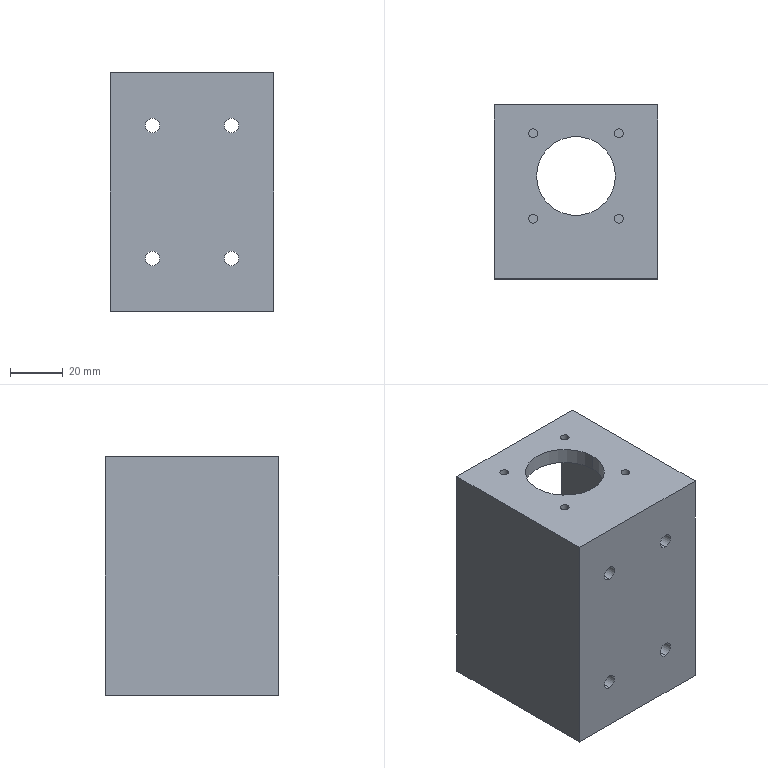Part | Creo | features CURVE 7, CUT 4, DATUM PLANE 3, PROTRUSION 2, CHAMFER 1, COORDINATE SYSTEM 1 | 1 solid | 45 faces | box 62 x 66 x 90.5 mm | volume 126268 mm3 | cylinder 26 | plane 19 | commonest cylinder face diameters 3.3 x8 5.5 x8 4.2 x6 30 x2 34 x2
STEP:
#1=CARTESIAN_POINT('',(0.,0.,0.));
#2=DIRECTION('',(0.,0.,1.));
#3=DIRECTION('',(1.,0.,0.));
#4=AXIS2_PLACEMENT_3D('',#1,#2,#3);
#5=CARTESIAN_POINT('',(31.,27.,0.));
#6=VERTEX_POINT('',#5);
#7=CARTESIAN_POINT('',(-31.,27.,0.));
#8=VERTEX_POINT('',#7);
#9=CARTESIAN_POINT('',(31.,27.,0.));
#10=DIRECTION('',(-1.,0.,0.));
#11=VECTOR('',#10,62.);
#12=LINE('',#9,#11);
#13=EDGE_CURVE('',#6,#8,#12,.T.);
#14=ORIENTED_EDGE('',*,*,#13,.T.);
#15=CARTESIAN_POINT('',(-31.,-39.,0.));
#16=VERTEX_POINT('',#15);
#17=CARTESIAN_POINT('',(-31.,27.,0.));
#18=DIRECTION('',(0.,-1.,0.));
#19=VECTOR('',#18,66.);
#20=LINE('',#17,#19);
#21=EDGE_CURVE('',#8,#16,#20,.T.);
#22=ORIENTED_EDGE('',*,*,#21,.T.);
#23=CARTESIAN_POINT('',(31.,-39.,0.));
#24=VERTEX_POINT('',#23);
#25=CARTESIAN_POINT('',(-31.,-39.,0.));
#26=DIRECTION('',(1.,0.,0.));
#27=VECTOR('',#26,62.);
#28=LINE('',#25,#27);
#29=EDGE_CURVE('',#16,#24,#28,.T.);
#30=ORIENTED_EDGE('',*,*,#29,.T.);
#31=CARTESIAN_POINT('',(31.,-39.,0.));
#32=DIRECTION('',(0.,1.,0.));
#33=VECTOR('',#32,66.);
#34=LINE('',#31,#33);
#35=EDGE_CURVE('',#24,#6,#34,.T.);
#36=ORIENTED_EDGE('',*,*,#35,.T.);
#37=EDGE_LOOP('',(#14,#22,#30,#36));
#38=FACE_OUTER_BOUND('',#37,.F.);
#39=CARTESIAN_POINT('',(0.,-17.,0.));
#40=VERTEX_POINT('',#39);
#41=CARTESIAN_POINT('',(0.,17.,0.));
#42=VERTEX_POINT('',#41);
#43=CARTESIAN_POINT('',(0.,0.,0.));
#44=DIRECTION('',(0.,0.,-1.));
#45=DIRECTION('',(0.,-1.,0.));
#46=AXIS2_PLACEMENT_3D('',#43,#44,#45);
#47=CIRCLE('',#46,17.);
#48=EDGE_CURVE('',#40,#42,#47,.T.);
#49=ORIENTED_EDGE('',*,*,#48,.T.);
#50=CARTESIAN_POINT('',(0.,0.,0.));
#51=DIRECTION('',(0.,0.,-1.));
#52=DIRECTION('',(0.,1.,0.));
#53=AXIS2_PLACEMENT_3D('',#50,#51,#52);
#54=CIRCLE('',#53,17.);
#55=EDGE_CURVE('',#42,#40,#54,.T.);
#56=ORIENTED_EDGE('',*,*,#55,.T.);
#57=EDGE_LOOP('',(#49,#56));
#58=FACE_BOUND('',#57,.F.);
#59=CARTESIAN_POINT('',(0.,18.9,0.));
#60=VERTEX_POINT('',#59);
#61=CARTESIAN_POINT('',(0.,23.1,0.));
#62=VERTEX_POINT('',#61);
#63=CARTESIAN_POINT('',(0.,21.,0.));
#64=DIRECTION('',(0.,0.,-1.));
#65=DIRECTION('',(0.,-1.,0.));
#66=AXIS2_PLACEMENT_3D('',#63,#64,#65);
#67=CIRCLE('',#66,2.1);
#68=EDGE_CURVE('',#60,#62,#67,.T.);
#69=ORIENTED_EDGE('',*,*,#68,.T.);
#70=CARTESIAN_POINT('',(0.,21.,0.));
#71=DIRECTION('',(0.,0.,-1.));
#72=DIRECTION('',(0.,1.,0.));
#73=AXIS2_PLACEMENT_3D('',#70,#71,#72);
#74=CIRCLE('',#73,2.1);
#75=EDGE_CURVE('',#62,#60,#74,.T.);
#76=ORIENTED_EDGE('',*,*,#75,.T.);
#77=EDGE_LOOP('',(#69,#76));
#78=FACE_BOUND('',#77,.F.);
#79=CARTESIAN_POINT('',(-18.187,-12.6,0.));
#80=VERTEX_POINT('',#79);
#81=CARTESIAN_POINT('',(-18.187,-8.4,0.));
#82=VERTEX_POINT('',#81);
#83=CARTESIAN_POINT('',(-18.187,-10.5,0.));
#84=DIRECTION('',(0.,0.,-1.));
#85=DIRECTION('',(0.,-1.,0.));
#86=AXIS2_PLACEMENT_3D('',#83,#84,#85);
#87=CIRCLE('',#86,2.1);
#88=EDGE_CURVE('',#80,#82,#87,.T.);
#89=ORIENTED_EDGE('',*,*,#88,.T.);
#90=CARTESIAN_POINT('',(-18.187,-10.5,0.));
#91=DIRECTION('',(0.,0.,-1.));
#92=DIRECTION('',(0.,1.,0.));
#93=AXIS2_PLACEMENT_3D('',#90,#91,#92);
#94=CIRCLE('',#93,2.1);
#95=EDGE_CURVE('',#82,#80,#94,.T.);
#96=ORIENTED_EDGE('',*,*,#95,.T.);
#97=EDGE_LOOP('',(#89,#96));
#98=FACE_BOUND('',#97,.F.);
#99=CARTESIAN_POINT('',(18.187,-12.6,0.));
#100=VERTEX_POINT('',#99);
#101=CARTESIAN_POINT('',(18.187,-8.4,0.));
#102=VERTEX_POINT('',#101);
#103=CARTESIAN_POINT('',(18.187,-10.5,0.));
#104=DIRECTION('',(0.,0.,-1.));
#105=DIRECTION('',(0.,-1.,0.));
#106=AXIS2_PLACEMENT_3D('',#103,#104,#105);
#107=CIRCLE('',#106,2.1);
#108=EDGE_CURVE('',#100,#102,#107,.T.);
#109=ORIENTED_EDGE('',*,*,#108,.T.);
#110=CARTESIAN_POINT('',(18.187,-10.5,0.));
#111=DIRECTION('',(0.,0.,-1.));
#112=DIRECTION('',(0.,1.,0.));
#113=AXIS2_PLACEMENT_3D('',#110,#111,#112);
#114=CIRCLE('',#113,2.1);
#115=EDGE_CURVE('',#102,#100,#114,.T.);
#116=ORIENTED_EDGE('',*,*,#115,.T.);
#117=EDGE_LOOP('',(#109,#116));
#118=FACE_BOUND('',#117,.F.);
#119=CARTESIAN_POINT('',(0.,0.,0.));
#120=DIRECTION('',(0.,0.,1.));
#121=DIRECTION('',(1.,0.,0.));
#122=AXIS2_PLACEMENT_3D('',#119,#120,#121);
#123=PLANE('',#122);
#124=ADVANCED_FACE('',(#38,#58,#78,#98,#118),#123,.F.);
#125=ORIENTED_EDGE('',*,*,#13,.F.);
#126=CARTESIAN_POINT('',(31.,27.,90.5));
#127=VERTEX_POINT('',#126);
#128=CARTESIAN_POINT('',(31.,27.,0.));
#129=DIRECTION('',(0.,0.,1.));
#130=VECTOR('',#129,90.5);
#131=LINE('',#128,#130);
#132=EDGE_CURVE('',#6,#127,#131,.T.);
#133=ORIENTED_EDGE('',*,*,#132,.T.);
#134=CARTESIAN_POINT('',(-31.,27.,90.5));
#135=VERTEX_POINT('',#134);
#136=CARTESIAN_POINT('',(31.,27.,90.5));
#137=DIRECTION('',(-1.,0.,0.));
#138=VECTOR('',#137,62.);
#139=LINE('',#136,#138);
#140=EDGE_CURVE('',#127,#135,#139,.T.);
#141=ORIENTED_EDGE('',*,*,#140,.T.);
#142=CARTESIAN_POINT('',(-31.,27.,0.));
#143=DIRECTION('',(0.,0.,1.));
#144=VECTOR('',#143,90.5);
#145=LINE('',#142,#144);
#146=EDGE_CURVE('',#8,#135,#145,.T.);
#147=ORIENTED_EDGE('',*,*,#146,.F.);
#148=EDGE_LOOP('',(#125,#133,#141,#147));
#149=FACE_OUTER_BOUND('',#148,.F.);
#150=CARTESIAN_POINT('',(-25.,27.,9.));
#151=VERTEX_POINT('',#150);
#152=CARTESIAN_POINT('',(-25.,27.,81.5));
#153=VERTEX_POINT('',#152);
#154=CARTESIAN_POINT('',(-25.,27.,9.));
#155=DIRECTION('',(0.,0.,1.));
#156=VECTOR('',#155,72.5);
#157=LINE('',#154,#156);
#158=EDGE_CURVE('',#151,#153,#157,.T.);
#159=ORIENTED_EDGE('',*,*,#158,.T.);
#160=CARTESIAN_POINT('',(-22.,27.,84.5));
#161=VERTEX_POINT('',#160);
#162=CARTESIAN_POINT('',(-22.,27.,84.5));
#163=DIRECTION('',(-0.7071,0.,-0.7071));
#164=VECTOR('',#163,4.243);
#165=LINE('',#162,#164);
#166=EDGE_CURVE('',#161,#153,#165,.T.);
#167=ORIENTED_EDGE('',*,*,#166,.F.);
#168=CARTESIAN_POINT('',(22.,27.,84.5));
#169=VERTEX_POINT('',#168);
#170=CARTESIAN_POINT('',(-22.,27.,84.5));
#171=DIRECTION('',(1.,0.,0.));
#172=VECTOR('',#171,44.);
#173=LINE('',#170,#172);
#174=EDGE_CURVE('',#161,#169,#173,.T.);
#175=ORIENTED_EDGE('',*,*,#174,.T.);
#176=CARTESIAN_POINT('',(25.,27.,81.5));
#177=VERTEX_POINT('',#176);
#178=CARTESIAN_POINT('',(25.,27.,81.5));
#179=DIRECTION('',(-0.7071,0.,0.7071));
#180=VECTOR('',#179,4.243);
#181=LINE('',#178,#180);
#182=EDGE_CURVE('',#177,#169,#181,.T.);
#183=ORIENTED_EDGE('',*,*,#182,.F.);
#184=CARTESIAN_POINT('',(25.,27.,9.));
#185=VERTEX_POINT('',#184);
#186=CARTESIAN_POINT('',(25.,27.,81.5));
#187=DIRECTION('',(0.,0.,-1.));
#188=VECTOR('',#187,72.5);
#189=LINE('',#186,#188);
#190=EDGE_CURVE('',#177,#185,#189,.T.);
#191=ORIENTED_EDGE('',*,*,#190,.T.);
#192=CARTESIAN_POINT('',(22.,27.,6.));
#193=VERTEX_POINT('',#192);
#194=CARTESIAN_POINT('',(22.,27.,6.));
#195=DIRECTION('',(0.7071,0.,0.7071));
#196=VECTOR('',#195,4.243);
#197=LINE('',#194,#196);
#198=EDGE_CURVE('',#193,#185,#197,.T.);
#199=ORIENTED_EDGE('',*,*,#198,.F.);
#200=CARTESIAN_POINT('',(-22.,27.,6.));
#201=VERTEX_POINT('',#200);
#202=CARTESIAN_POINT('',(22.,27.,6.));
#203=DIRECTION('',(-1.,0.,0.));
#204=VECTOR('',#203,44.);
#205=LINE('',#202,#204);
#206=EDGE_CURVE('',#193,#201,#205,.T.);
#207=ORIENTED_EDGE('',*,*,#206,.T.);
#208=CARTESIAN_POINT('',(-25.,27.,9.));
#209=DIRECTION('',(0.7071,0.,-0.7071));
#210=VECTOR('',#209,4.243);
#211=LINE('',#208,#210);
#212=EDGE_CURVE('',#151,#201,#211,.T.);
#213=ORIENTED_EDGE('',*,*,#212,.F.);
#214=EDGE_LOOP('',(#159,#167,#175,#183,#191,#199,#207,#213));
#215=FACE_BOUND('',#214,.F.);
#216=CARTESIAN_POINT('',(31.,27.,0.));
#217=DIRECTION('',(0.,1.,0.));
#218=DIRECTION('',(-1.,0.,0.));
#219=AXIS2_PLACEMENT_3D('',#216,#217,#218);
#220=PLANE('',#219);
#221=ADVANCED_FACE('',(#149,#215),#220,.T.);
#222=ORIENTED_EDGE('',*,*,#35,.F.);
#223=CARTESIAN_POINT('',(31.,-39.,90.5));
#224=VERTEX_POINT('',#223);
#225=CARTESIAN_POINT('',(31.,-39.,0.));
#226=DIRECTION('',(0.,0.,1.));
#227=VECTOR('',#226,90.5);
#228=LINE('',#225,#227);
#229=EDGE_CURVE('',#24,#224,#228,.T.);
#230=ORIENTED_EDGE('',*,*,#229,.T.);
#231=CARTESIAN_POINT('',(31.,-39.,90.5));
#232=DIRECTION('',(0.,1.,0.));
#233=VECTOR('',#232,66.);
#234=LINE('',#231,#233);
#235=EDGE_CURVE('',#224,#127,#234,.T.);
#236=ORIENTED_EDGE('',*,*,#235,.T.);
#237=ORIENTED_EDGE('',*,*,#132,.F.);
#238=EDGE_LOOP('',(#222,#230,#236,#237));
#239=FACE_OUTER_BOUND('',#238,.F.);
#240=CARTESIAN_POINT('',(31.,-39.,0.));
#241=DIRECTION('',(1.,0.,0.));
#242=DIRECTION('',(0.,1.,0.));
#243=AXIS2_PLACEMENT_3D('',#240,#241,#242);
#244=PLANE('',#243);
#245=ADVANCED_FACE('',(#239),#244,.T.);
#246=ORIENTED_EDGE('',*,*,#29,.F.);
#247=CARTESIAN_POINT('',(-31.,-39.,90.5));
#248=VERTEX_POINT('',#247);
#249=CARTESIAN_POINT('',(-31.,-39.,0.));
#250=DIRECTION('',(0.,0.,1.));
#251=VECTOR('',#250,90.5);
#252=LINE('',#249,#251);
#253=EDGE_CURVE('',#16,#248,#252,.T.);
#254=ORIENTED_EDGE('',*,*,#253,.T.);
#255=CARTESIAN_POINT('',(-31.,-39.,90.5));
#256=DIRECTION('',(1.,0.,0.));
#257=VECTOR('',#256,62.);
#258=LINE('',#255,#257);
#259=EDGE_CURVE('',#248,#224,#258,.T.);
#260=ORIENTED_EDGE('',*,*,#259,.T.);
#261=ORIENTED_EDGE('',*,*,#229,.F.);
#262=EDGE_LOOP('',(#246,#254,#260,#261));
#263=FACE_OUTER_BOUND('',#262,.F.);
#264=CARTESIAN_POINT('',(-15.,-39.,67.75));
#265=VERTEX_POINT('',#264);
#266=CARTESIAN_POINT('',(-15.,-39.,73.25));
#267=VERTEX_POINT('',#266);
#268=CARTESIAN_POINT('',(-15.,-39.,70.5));
#269=DIRECTION('',(0.,1.,0.));
#270=DIRECTION('',(0.,0.,-1.));
#271=AXIS2_PLACEMENT_3D('',#268,#269,#270);
#272=CIRCLE('',#271,2.75);
#273=EDGE_CURVE('',#265,#267,#272,.T.);
#274=ORIENTED_EDGE('',*,*,#273,.F.);
#275=CARTESIAN_POINT('',(-15.,-39.,70.5));
#276=DIRECTION('',(0.,1.,0.));
#277=DIRECTION('',(0.,0.,1.));
#278=AXIS2_PLACEMENT_3D('',#275,#276,#277);
#279=CIRCLE('',#278,2.75);
#280=EDGE_CURVE('',#267,#265,#279,.T.);
#281=ORIENTED_EDGE('',*,*,#280,.F.);
#282=EDGE_LOOP('',(#274,#281));
#283=FACE_BOUND('',#282,.F.);
#284=CARTESIAN_POINT('',(-15.,-39.,17.25));
#285=VERTEX_POINT('',#284);
#286=CARTESIAN_POINT('',(-15.,-39.,22.75));
#287=VERTEX_POINT('',#286);
#288=CARTESIAN_POINT('',(-15.,-39.,20.));
#289=DIRECTION('',(0.,1.,0.));
#290=DIRECTION('',(0.,0.,-1.));
#291=AXIS2_PLACEMENT_3D('',#288,#289,#290);
#292=CIRCLE('',#291,2.75);
#293=EDGE_CURVE('',#285,#287,#292,.T.);
#294=ORIENTED_EDGE('',*,*,#293,.F.);
#295=CARTESIAN_POINT('',(-15.,-39.,20.));
#296=DIRECTION('',(0.,1.,0.));
#297=DIRECTION('',(0.,0.,1.));
#298=AXIS2_PLACEMENT_3D('',#295,#296,#297);
#299=CIRCLE('',#298,2.75);
#300=EDGE_CURVE('',#287,#285,#299,.T.);
#301=ORIENTED_EDGE('',*,*,#300,.F.);
#302=EDGE_LOOP('',(#294,#301));
#303=FACE_BOUND('',#302,.F.);
#304=CARTESIAN_POINT('',(15.,-39.,17.25));
#305=VERTEX_POINT('',#304);
#306=CARTESIAN_POINT('',(15.,-39.,22.75));
#307=VERTEX_POINT('',#306);
#308=CARTESIAN_POINT('',(15.,-39.,20.));
#309=DIRECTION('',(0.,1.,0.));
#310=DIRECTION('',(0.,0.,-1.));
#311=AXIS2_PLACEMENT_3D('',#308,#309,#310);
#312=CIRCLE('',#311,2.75);
#313=EDGE_CURVE('',#305,#307,#312,.T.);
#314=ORIENTED_EDGE('',*,*,#313,.F.);
#315=CARTESIAN_POINT('',(15.,-39.,20.));
#316=DIRECTION('',(0.,1.,0.));
#317=DIRECTION('',(0.,0.,1.));
#318=AXIS2_PLACEMENT_3D('',#315,#316,#317);
#319=CIRCLE('',#318,2.75);
#320=EDGE_CURVE('',#307,#305,#319,.T.);
#321=ORIENTED_EDGE('',*,*,#320,.F.);
#322=EDGE_LOOP('',(#314,#321));
#323=FACE_BOUND('',#322,.F.);
#324=CARTESIAN_POINT('',(15.,-39.,67.75));
#325=VERTEX_POINT('',#324);
#326=CARTESIAN_POINT('',(15.,-39.,73.25));
#327=VERTEX_POINT('',#326);
#328=CARTESIAN_POINT('',(15.,-39.,70.5));
#329=DIRECTION('',(0.,1.,0.));
#330=DIRECTION('',(0.,0.,-1.));
#331=AXIS2_PLACEMENT_3D('',#328,#329,#330);
#332=CIRCLE('',#331,2.75);
#333=EDGE_CURVE('',#325,#327,#332,.T.);
#334=ORIENTED_EDGE('',*,*,#333,.F.);
#335=CARTESIAN_POINT('',(15.,-39.,70.5));
#336=DIRECTION('',(0.,1.,0.));
#337=DIRECTION('',(0.,0.,1.));
#338=AXIS2_PLACEMENT_3D('',#335,#336,#337);
#339=CIRCLE('',#338,2.75);
#340=EDGE_CURVE('',#327,#325,#339,.T.);
#341=ORIENTED_EDGE('',*,*,#340,.F.);
#342=EDGE_LOOP('',(#334,#341));
#343=FACE_BOUND('',#342,.F.);
#344=CARTESIAN_POINT('',(-31.,-39.,0.));
#345=DIRECTION('',(0.,-1.,0.));
#346=DIRECTION('',(1.,0.,0.));
#347=AXIS2_PLACEMENT_3D('',#344,#345,#346);
#348=PLANE('',#347);
#349=ADVANCED_FACE('',(#263,#283,#303,#323,#343),#348,.T.);
#350=ORIENTED_EDGE('',*,*,#21,.F.);
#351=ORIENTED_EDGE('',*,*,#146,.T.);
#352=CARTESIAN_POINT('',(-31.,27.,90.5));
#353=DIRECTION('',(0.,-1.,0.));
#354=VECTOR('',#353,66.);
#355=LINE('',#352,#354);
#356=EDGE_CURVE('',#135,#248,#355,.T.);
#357=ORIENTED_EDGE('',*,*,#356,.T.);
#358=ORIENTED_EDGE('',*,*,#253,.F.);
#359=EDGE_LOOP('',(#350,#351,#357,#358));
#360=FACE_OUTER_BOUND('',#359,.F.);
#361=CARTESIAN_POINT('',(-31.,27.,0.));
#362=DIRECTION('',(-1.,0.,0.));
#363=DIRECTION('',(0.,-1.,0.));
#364=AXIS2_PLACEMENT_3D('',#361,#362,#363);
#365=PLANE('',#364);
#366=ADVANCED_FACE('',(#360),#365,.T.);
#367=ORIENTED_EDGE('',*,*,#140,.F.);
#368=ORIENTED_EDGE('',*,*,#235,.F.);
#369=ORIENTED_EDGE('',*,*,#259,.F.);
#370=ORIENTED_EDGE('',*,*,#356,.F.);
#371=EDGE_LOOP('',(#367,#368,#369,#370));
#372=FACE_OUTER_BOUND('',#371,.F.);
#373=CARTESIAN_POINT('',(-14.61,16.26,90.5));
#374=VERTEX_POINT('',#373);
#375=CARTESIAN_POINT('',(-17.91,16.26,90.5));
#376=VERTEX_POINT('',#375);
#377=CARTESIAN_POINT('',(-16.26,16.26,90.5));
#378=DIRECTION('',(0.,0.,-1.));
#379=DIRECTION('',(1.,0.,0.));
#380=AXIS2_PLACEMENT_3D('',#377,#378,#379);
#381=CIRCLE('',#380,1.65);
#382=EDGE_CURVE('',#374,#376,#381,.T.);
#383=ORIENTED_EDGE('',*,*,#382,.F.);
#384=CARTESIAN_POINT('',(-16.26,16.26,90.5));
#385=DIRECTION('',(0.,0.,-1.));
#386=DIRECTION('',(-1.,0.,0.));
#387=AXIS2_PLACEMENT_3D('',#384,#385,#386);
#388=CIRCLE('',#387,1.65);
#389=EDGE_CURVE('',#376,#374,#388,.T.);
#390=ORIENTED_EDGE('',*,*,#389,.F.);
#391=EDGE_LOOP('',(#383,#390));
#392=FACE_BOUND('',#391,.F.);
#393=CARTESIAN_POINT('',(17.91,16.26,90.5));
#394=VERTEX_POINT('',#393);
#395=CARTESIAN_POINT('',(14.61,16.26,90.5));
#396=VERTEX_POINT('',#395);
#397=CARTESIAN_POINT('',(16.26,16.26,90.5));
#398=DIRECTION('',(0.,0.,-1.));
#399=DIRECTION('',(1.,0.,0.));
#400=AXIS2_PLACEMENT_3D('',#397,#398,#399);
#401=CIRCLE('',#400,1.65);
#402=EDGE_CURVE('',#394,#396,#401,.T.);
#403=ORIENTED_EDGE('',*,*,#402,.F.);
#404=CARTESIAN_POINT('',(16.26,16.26,90.5));
#405=DIRECTION('',(0.,0.,-1.));
#406=DIRECTION('',(-1.,0.,0.));
#407=AXIS2_PLACEMENT_3D('',#404,#405,#406);
#408=CIRCLE('',#407,1.65);
#409=EDGE_CURVE('',#396,#394,#408,.T.);
#410=ORIENTED_EDGE('',*,*,#409,.F.);
#411=EDGE_LOOP('',(#403,#410));
#412=FACE_BOUND('',#411,.F.);
#413=CARTESIAN_POINT('',(17.91,-16.26,90.5));
#414=VERTEX_POINT('',#413);
#415=CARTESIAN_POINT('',(14.61,-16.26,90.5));
#416=VERTEX_POINT('',#415);
#417=CARTESIAN_POINT('',(16.26,-16.26,90.5));
#418=DIRECTION('',(0.,0.,-1.));
#419=DIRECTION('',(1.,0.,0.));
#420=AXIS2_PLACEMENT_3D('',#417,#418,#419);
#421=CIRCLE('',#420,1.65);
#422=EDGE_CURVE('',#414,#416,#421,.T.);
#423=ORIENTED_EDGE('',*,*,#422,.F.);
#424=CARTESIAN_POINT('',(16.26,-16.26,90.5));
#425=DIRECTION('',(0.,0.,-1.));
#426=DIRECTION('',(-1.,0.,0.));
#427=AXIS2_PLACEMENT_3D('',#424,#425,#426);
#428=CIRCLE('',#427,1.65);
#429=EDGE_CURVE('',#416,#414,#428,.T.);
#430=ORIENTED_EDGE('',*,*,#429,.F.);
#431=EDGE_LOOP('',(#423,#430));
#432=FACE_BOUND('',#431,.F.);
#433=CARTESIAN_POINT('',(-14.61,-16.26,90.5));
#434=VERTEX_POINT('',#433);
#435=CARTESIAN_POINT('',(-17.91,-16.26,90.5));
#436=VERTEX_POINT('',#435);
#437=CARTESIAN_POINT('',(-16.26,-16.26,90.5));
#438=DIRECTION('',(0.,0.,-1.));
#439=DIRECTION('',(1.,0.,0.));
#440=AXIS2_PLACEMENT_3D('',#437,#438,#439);
#441=CIRCLE('',#440,1.65);
#442=EDGE_CURVE('',#434,#436,#441,.T.);
#443=ORIENTED_EDGE('',*,*,#442,.F.);
#444=CARTESIAN_POINT('',(-16.26,-16.26,90.5));
#445=DIRECTION('',(0.,0.,-1.));
#446=DIRECTION('',(-1.,0.,0.));
#447=AXIS2_PLACEMENT_3D('',#444,#445,#446);
#448=CIRCLE('',#447,1.65);
#449=EDGE_CURVE('',#436,#434,#448,.T.);
#450=ORIENTED_EDGE('',*,*,#449,.F.);
#451=EDGE_LOOP('',(#443,#450));
#452=FACE_BOUND('',#451,.F.);
#453=CARTESIAN_POINT('',(15.,0.,90.5));
#454=VERTEX_POINT('',#453);
#455=CARTESIAN_POINT('',(-15.,0.,90.5));
#456=VERTEX_POINT('',#455);
#457=CARTESIAN_POINT('',(0.,0.,90.5));
#458=DIRECTION('',(0.,0.,-1.));
#459=DIRECTION('',(1.,0.,0.));
#460=AXIS2_PLACEMENT_3D('',#457,#458,#459);
#461=CIRCLE('',#460,15.);
#462=EDGE_CURVE('',#454,#456,#461,.T.);
#463=ORIENTED_EDGE('',*,*,#462,.F.);
#464=CARTESIAN_POINT('',(0.,0.,90.5));
#465=DIRECTION('',(0.,0.,-1.));
#466=DIRECTION('',(-1.,0.,0.));
#467=AXIS2_PLACEMENT_3D('',#464,#465,#466);
#468=CIRCLE('',#467,15.);
#469=EDGE_CURVE('',#456,#454,#468,.T.);
#470=ORIENTED_EDGE('',*,*,#469,.F.);
#471=EDGE_LOOP('',(#463,#470));
#472=FACE_BOUND('',#471,.F.);
#473=CARTESIAN_POINT('',(0.,0.,90.5));
#474=DIRECTION('',(0.,0.,1.));
#475=DIRECTION('',(1.,0.,0.));
#476=AXIS2_PLACEMENT_3D('',#473,#474,#475);
#477=PLANE('',#476);
#478=ADVANCED_FACE('',(#372,#392,#412,#432,#452,#472),#477,.T.);
#479=CARTESIAN_POINT('',(-15.,0.,84.5));
#480=VERTEX_POINT('',#479);
#481=CARTESIAN_POINT('',(15.,0.,84.5));
#482=VERTEX_POINT('',#481);
#483=CARTESIAN_POINT('',(0.,0.,84.5));
#484=DIRECTION('',(0.,0.,1.));
#485=DIRECTION('',(-1.,0.,0.));
#486=AXIS2_PLACEMENT_3D('',#483,#484,#485);
#487=CIRCLE('',#486,15.);
#488=EDGE_CURVE('',#480,#482,#487,.T.);
#489=ORIENTED_EDGE('',*,*,#488,.T.);
#490=CARTESIAN_POINT('',(15.,0.,84.5));
#491=DIRECTION('',(0.,0.,1.));
#492=VECTOR('',#491,6.);
#493=LINE('',#490,#492);
#494=EDGE_CURVE('',#482,#454,#493,.T.);
#495=ORIENTED_EDGE('',*,*,#494,.T.);
#496=ORIENTED_EDGE('',*,*,#462,.T.);
#497=CARTESIAN_POINT('',(-15.,0.,84.5));
#498=DIRECTION('',(0.,0.,1.));
#499=VECTOR('',#498,6.);
#500=LINE('',#497,#499);
#501=EDGE_CURVE('',#480,#456,#500,.T.);
#502=ORIENTED_EDGE('',*,*,#501,.F.);
#503=EDGE_LOOP('',(#489,#495,#496,#502));
#504=FACE_OUTER_BOUND('',#503,.F.);
#505=CARTESIAN_POINT('',(0.,0.,0.));
#506=DIRECTION('',(0.,0.,1.));
#507=DIRECTION('',(1.,0.,0.));
#508=AXIS2_PLACEMENT_3D('',#505,#506,#507);
#509=CYLINDRICAL_SURFACE('',#508,15.);
#510=ADVANCED_FACE('',(#504),#509,.F.);
#511=CARTESIAN_POINT('',(22.,-30.,84.5));
#512=VERTEX_POINT('',#511);
#513=CARTESIAN_POINT('',(22.,27.,84.5));
#514=DIRECTION('',(0.,-1.,0.));
#515=VECTOR('',#514,57.);
#516=LINE('',#513,#515);
#517=EDGE_CURVE('',#169,#512,#516,.T.);
#518=ORIENTED_EDGE('',*,*,#517,.F.);
#519=ORIENTED_EDGE('',*,*,#174,.F.);
#520=CARTESIAN_POINT('',(-22.,-30.,84.5));
#521=VERTEX_POINT('',#520);
#522=CARTESIAN_POINT('',(-22.,27.,84.5));
#523=DIRECTION('',(0.,-1.,0.));
#524=VECTOR('',#523,57.);
#525=LINE('',#522,#524);
#526=EDGE_CURVE('',#161,#521,#525,.T.);
#527=ORIENTED_EDGE('',*,*,#526,.T.);
#528=CARTESIAN_POINT('',(22.,-30.,84.5));
#529=DIRECTION('',(-1.,0.,0.));
#530=VECTOR('',#529,44.);
#531=LINE('',#528,#530);
#532=EDGE_CURVE('',#512,#521,#531,.T.);
#533=ORIENTED_EDGE('',*,*,#532,.F.);
#534=EDGE_LOOP('',(#518,#519,#527,#533));
#535=FACE_OUTER_BOUND('',#534,.F.);
#536=CARTESIAN_POINT('',(-17.91,16.26,84.5));
#537=VERTEX_POINT('',#536);
#538=CARTESIAN_POINT('',(-14.61,16.26,84.5));
#539=VERTEX_POINT('',#538);
#540=CARTESIAN_POINT('',(-16.26,16.26,84.5));
#541=DIRECTION('',(0.,0.,1.));
#542=DIRECTION('',(-1.,0.,0.));
#543=AXIS2_PLACEMENT_3D('',#540,#541,#542);
#544=CIRCLE('',#543,1.65);
#545=EDGE_CURVE('',#537,#539,#544,.T.);
#546=ORIENTED_EDGE('',*,*,#545,.F.);
#547=CARTESIAN_POINT('',(-16.26,16.26,84.5));
#548=DIRECTION('',(0.,0.,1.));
#549=DIRECTION('',(1.,0.,0.));
#550=AXIS2_PLACEMENT_3D('',#547,#548,#549);
#551=CIRCLE('',#550,1.65);
#552=EDGE_CURVE('',#539,#537,#551,.T.);
#553=ORIENTED_EDGE('',*,*,#552,.F.);
#554=EDGE_LOOP('',(#546,#553));
#555=FACE_BOUND('',#554,.F.);
#556=CARTESIAN_POINT('',(14.61,16.26,84.5));
#557=VERTEX_POINT('',#556);
#558=CARTESIAN_POINT('',(17.91,16.26,84.5));
#559=VERTEX_POINT('',#558);
#560=CARTESIAN_POINT('',(16.26,16.26,84.5));
#561=DIRECTION('',(0.,0.,1.));
#562=DIRECTION('',(-1.,0.,0.));
#563=AXIS2_PLACEMENT_3D('',#560,#561,#562);
#564=CIRCLE('',#563,1.65);
#565=EDGE_CURVE('',#557,#559,#564,.T.);
#566=ORIENTED_EDGE('',*,*,#565,.F.);
#567=CARTESIAN_POINT('',(16.26,16.26,84.5));
#568=DIRECTION('',(0.,0.,1.));
#569=DIRECTION('',(1.,0.,0.));
#570=AXIS2_PLACEMENT_3D('',#567,#568,#569);
#571=CIRCLE('',#570,1.65);
#572=EDGE_CURVE('',#559,#557,#571,.T.);
#573=ORIENTED_EDGE('',*,*,#572,.F.);
#574=EDGE_LOOP('',(#566,#573));
#575=FACE_BOUND('',#574,.F.);
#576=CARTESIAN_POINT('',(14.61,-16.26,84.5));
#577=VERTEX_POINT('',#576);
#578=CARTESIAN_POINT('',(17.91,-16.26,84.5));
#579=VERTEX_POINT('',#578);
#580=CARTESIAN_POINT('',(16.26,-16.26,84.5));
#581=DIRECTION('',(0.,0.,1.));
#582=DIRECTION('',(-1.,0.,0.));
#583=AXIS2_PLACEMENT_3D('',#580,#581,#582);
#584=CIRCLE('',#583,1.65);
#585=EDGE_CURVE('',#577,#579,#584,.T.);
#586=ORIENTED_EDGE('',*,*,#585,.F.);
#587=CARTESIAN_POINT('',(16.26,-16.26,84.5));
#588=DIRECTION('',(0.,0.,1.));
#589=DIRECTION('',(1.,0.,0.));
#590=AXIS2_PLACEMENT_3D('',#587,#588,#589);
#591=CIRCLE('',#590,1.65);
#592=EDGE_CURVE('',#579,#577,#591,.T.);
#593=ORIENTED_EDGE('',*,*,#592,.F.);
#594=EDGE_LOOP('',(#586,#593));
#595=FACE_BOUND('',#594,.F.);
#596=CARTESIAN_POINT('',(-17.91,-16.26,84.5));
#597=VERTEX_POINT('',#596);
#598=CARTESIAN_POINT('',(-14.61,-16.26,84.5));
#599=VERTEX_POINT('',#598);
#600=CARTESIAN_POINT('',(-16.26,-16.26,84.5));
#601=DIRECTION('',(0.,0.,1.));
#602=DIRECTION('',(-1.,0.,0.));
#603=AXIS2_PLACEMENT_3D('',#600,#601,#602);
#604=CIRCLE('',#603,1.65);
#605=EDGE_CURVE('',#597,#599,#604,.T.);
#606=ORIENTED_EDGE('',*,*,#605,.F.);
#607=CARTESIAN_POINT('',(-16.26,-16.26,84.5));
#608=DIRECTION('',(0.,0.,1.));
#609=DIRECTION('',(1.,0.,0.));
#610=AXIS2_PLACEMENT_3D('',#607,#608,#609);
#611=CIRCLE('',#610,1.65);
#612=EDGE_CURVE('',#599,#597,#611,.T.);
#613=ORIENTED_EDGE('',*,*,#612,.F.);
#614=EDGE_LOOP('',(#606,#613));
#615=FACE_BOUND('',#614,.F.);
#616=ORIENTED_EDGE('',*,*,#488,.F.);
#617=CARTESIAN_POINT('',(0.,0.,84.5));
#618=DIRECTION('',(0.,0.,1.));
#619=DIRECTION('',(1.,0.,0.));
#620=AXIS2_PLACEMENT_3D('',#617,#618,#619);
#621=CIRCLE('',#620,15.);
#622=EDGE_CURVE('',#482,#480,#621,.T.);
#623=ORIENTED_EDGE('',*,*,#622,.F.);
#624=EDGE_LOOP('',(#616,#623));
#625=FACE_BOUND('',#624,.F.);
#626=CARTESIAN_POINT('',(-25.,27.,84.5));
#627=DIRECTION('',(0.,0.,1.));
#628=DIRECTION('',(1.,0.,0.));
#629=AXIS2_PLACEMENT_3D('',#626,#627,#628);
#630=PLANE('',#629);
#631=ADVANCED_FACE('',(#535,#555,#575,#595,#615,#625),#630,.F.);
#632=ORIENTED_EDGE('',*,*,#622,.T.);
#633=ORIENTED_EDGE('',*,*,#501,.T.);
#634=ORIENTED_EDGE('',*,*,#469,.T.);
#635=ORIENTED_EDGE('',*,*,#494,.F.);
#636=EDGE_LOOP('',(#632,#633,#634,#635));
#637=FACE_OUTER_BOUND('',#636,.F.);
#638=CARTESIAN_POINT('',(0.,0.,0.));
#639=DIRECTION('',(0.,0.,1.));
#640=DIRECTION('',(1.,0.,0.));
#641=AXIS2_PLACEMENT_3D('',#638,#639,#640);
#642=CYLINDRICAL_SURFACE('',#641,15.);
#643=ADVANCED_FACE('',(#637),#642,.F.);
#644=ORIENTED_EDGE('',*,*,#545,.T.);
#645=CARTESIAN_POINT('',(-14.61,16.26,84.5));
#646=DIRECTION('',(0.,0.,1.));
#647=VECTOR('',#646,6.);
#648=LINE('',#645,#647);
#649=EDGE_CURVE('',#539,#374,#648,.T.);
#650=ORIENTED_EDGE('',*,*,#649,.T.);
#651=ORIENTED_EDGE('',*,*,#382,.T.);
#652=CARTESIAN_POINT('',(-17.91,16.26,84.5));
#653=DIRECTION('',(0.,0.,1.));
#654=VECTOR('',#653,6.);
#655=LINE('',#652,#654);
#656=EDGE_CURVE('',#537,#376,#655,.T.);
#657=ORIENTED_EDGE('',*,*,#656,.F.);
#658=EDGE_LOOP('',(#644,#650,#651,#657));
#659=FACE_OUTER_BOUND('',#658,.F.);
#660=CARTESIAN_POINT('',(-16.26,16.26,0.));
#661=DIRECTION('',(0.,0.,1.));
#662=DIRECTION('',(1.,0.,0.));
#663=AXIS2_PLACEMENT_3D('',#660,#661,#662);
#664=CYLINDRICAL_SURFACE('',#663,1.65);
#665=ADVANCED_FACE('',(#659),#664,.F.);
#666=ORIENTED_EDGE('',*,*,#552,.T.);
#667=ORIENTED_EDGE('',*,*,#656,.T.);
#668=ORIENTED_EDGE('',*,*,#389,.T.);
#669=ORIENTED_EDGE('',*,*,#649,.F.);
#670=EDGE_LOOP('',(#666,#667,#668,#669));
#671=FACE_OUTER_BOUND('',#670,.F.);
#672=CARTESIAN_POINT('',(-16.26,16.26,0.));
#673=DIRECTION('',(0.,0.,1.));
#674=DIRECTION('',(1.,0.,0.));
#675=AXIS2_PLACEMENT_3D('',#672,#673,#674);
#676=CYLINDRICAL_SURFACE('',#675,1.65);
#677=ADVANCED_FACE('',(#671),#676,.F.);
#678=ORIENTED_EDGE('',*,*,#565,.T.);
#679=CARTESIAN_POINT('',(17.91,16.26,84.5));
#680=DIRECTION('',(0.,0.,1.));
#681=VECTOR('',#680,6.);
#682=LINE('',#679,#681);
#683=EDGE_CURVE('',#559,#394,#682,.T.);
#684=ORIENTED_EDGE('',*,*,#683,.T.);
#685=ORIENTED_EDGE('',*,*,#402,.T.);
#686=CARTESIAN_POINT('',(14.61,16.26,84.5));
#687=DIRECTION('',(0.,0.,1.));
#688=VECTOR('',#687,6.);
#689=LINE('',#686,#688);
#690=EDGE_CURVE('',#557,#396,#689,.T.);
#691=ORIENTED_EDGE('',*,*,#690,.F.);
#692=EDGE_LOOP('',(#678,#684,#685,#691));
#693=FACE_OUTER_BOUND('',#692,.F.);
#694=CARTESIAN_POINT('',(16.26,16.26,0.));
#695=DIRECTION('',(0.,0.,1.));
#696=DIRECTION('',(1.,0.,0.));
#697=AXIS2_PLACEMENT_3D('',#694,#695,#696);
#698=CYLINDRICAL_SURFACE('',#697,1.65);
#699=ADVANCED_FACE('',(#693),#698,.F.);
#700=ORIENTED_EDGE('',*,*,#572,.T.);
#701=ORIENTED_EDGE('',*,*,#690,.T.);
#702=ORIENTED_EDGE('',*,*,#409,.T.);
#703=ORIENTED_EDGE('',*,*,#683,.F.);
#704=EDGE_LOOP('',(#700,#701,#702,#703));
#705=FACE_OUTER_BOUND('',#704,.F.);
#706=CARTESIAN_POINT('',(16.26,16.26,0.));
#707=DIRECTION('',(0.,0.,1.));
#708=DIRECTION('',(1.,0.,0.));
#709=AXIS2_PLACEMENT_3D('',#706,#707,#708);
#710=CYLINDRICAL_SURFACE('',#709,1.65);
#711=ADVANCED_FACE('',(#705),#710,.F.);
#712=ORIENTED_EDGE('',*,*,#585,.T.);
#713=CARTESIAN_POINT('',(17.91,-16.26,84.5));
#714=DIRECTION('',(0.,0.,1.));
#715=VECTOR('',#714,6.);
#716=LINE('',#713,#715);
#717=EDGE_CURVE('',#579,#414,#716,.T.);
#718=ORIENTED_EDGE('',*,*,#717,.T.);
#719=ORIENTED_EDGE('',*,*,#422,.T.);
#720=CARTESIAN_POINT('',(14.61,-16.26,84.5));
#721=DIRECTION('',(0.,0.,1.));
#722=VECTOR('',#721,6.);
#723=LINE('',#720,#722);
#724=EDGE_CURVE('',#577,#416,#723,.T.);
#725=ORIENTED_EDGE('',*,*,#724,.F.);
#726=EDGE_LOOP('',(#712,#718,#719,#725));
#727=FACE_OUTER_BOUND('',#726,.F.);
#728=CARTESIAN_POINT('',(16.26,-16.26,0.));
#729=DIRECTION('',(0.,0.,1.));
#730=DIRECTION('',(1.,0.,0.));
#731=AXIS2_PLACEMENT_3D('',#728,#729,#730);
#732=CYLINDRICAL_SURFACE('',#731,1.65);
#733=ADVANCED_FACE('',(#727),#732,.F.);
#734=ORIENTED_EDGE('',*,*,#592,.T.);
#735=ORIENTED_EDGE('',*,*,#724,.T.);
#736=ORIENTED_EDGE('',*,*,#429,.T.);
#737=ORIENTED_EDGE('',*,*,#717,.F.);
#738=EDGE_LOOP('',(#734,#735,#736,#737));
#739=FACE_OUTER_BOUND('',#738,.F.);
#740=CARTESIAN_POINT('',(16.26,-16.26,0.));
#741=DIRECTION('',(0.,0.,1.));
#742=DIRECTION('',(1.,0.,0.));
#743=AXIS2_PLACEMENT_3D('',#740,#741,#742);
#744=CYLINDRICAL_SURFACE('',#743,1.65);
#745=ADVANCED_FACE('',(#739),#744,.F.);
#746=ORIENTED_EDGE('',*,*,#605,.T.);
#747=CARTESIAN_POINT('',(-14.61,-16.26,84.5));
#748=DIRECTION('',(0.,0.,1.));
#749=VECTOR('',#748,6.);
#750=LINE('',#747,#749);
#751=EDGE_CURVE('',#599,#434,#750,.T.);
#752=ORIENTED_EDGE('',*,*,#751,.T.);
#753=ORIENTED_EDGE('',*,*,#442,.T.);
#754=CARTESIAN_POINT('',(-17.91,-16.26,84.5));
#755=DIRECTION('',(0.,0.,1.));
#756=VECTOR('',#755,6.);
#757=LINE('',#754,#756);
#758=EDGE_CURVE('',#597,#436,#757,.T.);
#759=ORIENTED_EDGE('',*,*,#758,.F.);
#760=EDGE_LOOP('',(#746,#752,#753,#759));
#761=FACE_OUTER_BOUND('',#760,.F.);
#762=CARTESIAN_POINT('',(-16.26,-16.26,0.));
#763=DIRECTION('',(0.,0.,1.));
#764=DIRECTION('',(1.,0.,0.));
#765=AXIS2_PLACEMENT_3D('',#762,#763,#764);
#766=CYLINDRICAL_SURFACE('',#765,1.65);
#767=ADVANCED_FACE('',(#761),#766,.F.);
#768=ORIENTED_EDGE('',*,*,#612,.T.);
#769=ORIENTED_EDGE('',*,*,#758,.T.);
#770=ORIENTED_EDGE('',*,*,#449,.T.);
#771=ORIENTED_EDGE('',*,*,#751,.F.);
#772=EDGE_LOOP('',(#768,#769,#770,#771));
#773=FACE_OUTER_BOUND('',#772,.F.);
#774=CARTESIAN_POINT('',(-16.26,-16.26,0.));
#775=DIRECTION('',(0.,0.,1.));
#776=DIRECTION('',(1.,0.,0.));
#777=AXIS2_PLACEMENT_3D('',#774,#775,#776);
#778=CYLINDRICAL_SURFACE('',#777,1.65);
#779=ADVANCED_FACE('',(#773),#778,.F.);
#780=ORIENTED_EDGE('',*,*,#517,.T.);
#781=CARTESIAN_POINT('',(23.5,-31.5,83.));
#782=VERTEX_POINT('',#781);
#783=CARTESIAN_POINT('',(23.5,-31.5,83.));
#784=DIRECTION('',(-0.5774,0.5774,0.5774));
#785=VECTOR('',#784,2.598);
#786=LINE('',#783,#785);
#787=EDGE_CURVE('',#782,#512,#786,.T.);
#788=ORIENTED_EDGE('',*,*,#787,.F.);
#789=CARTESIAN_POINT('',(25.,-30.,81.5));
#790=VERTEX_POINT('',#789);
#791=CARTESIAN_POINT('',(25.,-30.,81.5));
#792=DIRECTION('',(-0.5774,-0.5774,0.5774));
#793=VECTOR('',#792,2.598);
#794=LINE('',#791,#793);
#795=EDGE_CURVE('',#790,#782,#794,.T.);
#796=ORIENTED_EDGE('',*,*,#795,.F.);
#797=CARTESIAN_POINT('',(25.,27.,81.5));
#798=DIRECTION('',(0.,-1.,0.));
#799=VECTOR('',#798,57.);
#800=LINE('',#797,#799);
#801=EDGE_CURVE('',#177,#790,#800,.T.);
#802=ORIENTED_EDGE('',*,*,#801,.F.);
#803=ORIENTED_EDGE('',*,*,#182,.T.);
#804=EDGE_LOOP('',(#780,#788,#796,#802,#803));
#805=FACE_OUTER_BOUND('',#804,.F.);
#806=CARTESIAN_POINT('',(23.5,-3.,83.));
#807=DIRECTION('',(-0.7071,0.,-0.7071));
#808=DIRECTION('',(0.7071,0.,-0.7071));
#809=AXIS2_PLACEMENT_3D('',#806,#807,#808);
#810=PLANE('',#809);
#811=ADVANCED_FACE('',(#805),#810,.T.);
#812=ORIENTED_EDGE('',*,*,#532,.T.);
#813=CARTESIAN_POINT('',(-23.5,-31.5,83.));
#814=VERTEX_POINT('',#813);
#815=CARTESIAN_POINT('',(-22.,-30.,84.5));
#816=DIRECTION('',(-0.5774,-0.5774,-0.5774));
#817=VECTOR('',#816,2.598);
#818=LINE('',#815,#817);
#819=EDGE_CURVE('',#521,#814,#818,.T.);
#820=ORIENTED_EDGE('',*,*,#819,.T.);
#821=CARTESIAN_POINT('',(-22.,-33.,81.5));
#822=VERTEX_POINT('',#821);
#823=CARTESIAN_POINT('',(-22.,-33.,81.5));
#824=DIRECTION('',(-0.5774,0.5774,0.5774));
#825=VECTOR('',#824,2.598);
#826=LINE('',#823,#825);
#827=EDGE_CURVE('',#822,#814,#826,.T.);
#828=ORIENTED_EDGE('',*,*,#827,.F.);
#829=CARTESIAN_POINT('',(22.,-33.,81.5));
#830=VERTEX_POINT('',#829);
#831=CARTESIAN_POINT('',(22.,-33.,81.5));
#832=DIRECTION('',(-1.,0.,0.));
#833=VECTOR('',#832,44.);
#834=LINE('',#831,#833);
#835=EDGE_CURVE('',#830,#822,#834,.T.);
#836=ORIENTED_EDGE('',*,*,#835,.F.);
#837=CARTESIAN_POINT('',(22.,-33.,81.5));
#838=DIRECTION('',(0.5774,0.5774,0.5774));
#839=VECTOR('',#838,2.598);
#840=LINE('',#837,#839);
#841=EDGE_CURVE('',#830,#782,#840,.T.);
#842=ORIENTED_EDGE('',*,*,#841,.T.);
#843=ORIENTED_EDGE('',*,*,#787,.T.);
#844=EDGE_LOOP('',(#812,#820,#828,#836,#842,#843));
#845=FACE_OUTER_BOUND('',#844,.F.);
#846=CARTESIAN_POINT('',(0.,-31.5,83.));
#847=DIRECTION('',(0.,0.7071,-0.7071));
#848=DIRECTION('',(0.,-0.7071,-0.7071));
#849=AXIS2_PLACEMENT_3D('',#846,#847,#848);
#850=PLANE('',#849);
#851=ADVANCED_FACE('',(#845),#850,.T.);
#852=CARTESIAN_POINT('',(-25.,-30.,81.5));
#853=VERTEX_POINT('',#852);
#854=CARTESIAN_POINT('',(-25.,27.,81.5));
#855=DIRECTION('',(0.,-1.,0.));
#856=VECTOR('',#855,57.);
#857=LINE('',#854,#856);
#858=EDGE_CURVE('',#153,#853,#857,.T.);
#859=ORIENTED_EDGE('',*,*,#858,.T.);
#860=CARTESIAN_POINT('',(-23.5,-31.5,83.));
#861=DIRECTION('',(-0.5774,0.5774,-0.5774));
#862=VECTOR('',#861,2.598);
#863=LINE('',#860,#862);
#864=EDGE_CURVE('',#814,#853,#863,.T.);
#865=ORIENTED_EDGE('',*,*,#864,.F.);
#866=ORIENTED_EDGE('',*,*,#819,.F.);
#867=ORIENTED_EDGE('',*,*,#526,.F.);
#868=ORIENTED_EDGE('',*,*,#166,.T.);
#869=EDGE_LOOP('',(#859,#865,#866,#867,#868));
#870=FACE_OUTER_BOUND('',#869,.F.);
#871=CARTESIAN_POINT('',(-23.5,-3.,83.));
#872=DIRECTION('',(0.7071,0.,-0.7071));
#873=DIRECTION('',(0.7071,0.,0.7071));
#874=AXIS2_PLACEMENT_3D('',#871,#872,#873);
#875=PLANE('',#874);
#876=ADVANCED_FACE('',(#870),#875,.T.);
#877=CARTESIAN_POINT('',(-25.,-30.,9.));
#878=VERTEX_POINT('',#877);
#879=CARTESIAN_POINT('',(-25.,-30.,81.5));
#880=DIRECTION('',(0.,0.,-1.));
#881=VECTOR('',#880,72.5);
#882=LINE('',#879,#881);
#883=EDGE_CURVE('',#853,#878,#882,.T.);
#884=ORIENTED_EDGE('',*,*,#883,.F.);
#885=ORIENTED_EDGE('',*,*,#858,.F.);
#886=ORIENTED_EDGE('',*,*,#158,.F.);
#887=CARTESIAN_POINT('',(-25.,27.,9.));
#888=DIRECTION('',(0.,-1.,0.));
#889=VECTOR('',#888,57.);
#890=LINE('',#887,#889);
#891=EDGE_CURVE('',#151,#878,#890,.T.);
#892=ORIENTED_EDGE('',*,*,#891,.T.);
#893=EDGE_LOOP('',(#884,#885,#886,#892));
#894=FACE_OUTER_BOUND('',#893,.F.);
#895=CARTESIAN_POINT('',(-25.,27.,6.));
#896=DIRECTION('',(-1.,0.,0.));
#897=DIRECTION('',(0.,0.,1.));
#898=AXIS2_PLACEMENT_3D('',#895,#896,#897);
#899=PLANE('',#898);
#900=ADVANCED_FACE('',(#894),#899,.F.);
#901=CARTESIAN_POINT('',(-22.,-33.,9.));
#902=VERTEX_POINT('',#901);
#903=CARTESIAN_POINT('',(-22.,-33.,81.5));
#904=DIRECTION('',(0.,0.,-1.));
#905=VECTOR('',#904,72.5);
#906=LINE('',#903,#905);
#907=EDGE_CURVE('',#822,#902,#906,.T.);
#908=ORIENTED_EDGE('',*,*,#907,.F.);
#909=ORIENTED_EDGE('',*,*,#827,.T.);
#910=ORIENTED_EDGE('',*,*,#864,.T.);
#911=ORIENTED_EDGE('',*,*,#883,.T.);
#912=CARTESIAN_POINT('',(-23.5,-31.5,7.5));
#913=VERTEX_POINT('',#912);
#914=CARTESIAN_POINT('',(-25.,-30.,9.));
#915=DIRECTION('',(0.5774,-0.5774,-0.5774));
#916=VECTOR('',#915,2.598);
#917=LINE('',#914,#916);
#918=EDGE_CURVE('',#878,#913,#917,.T.);
#919=ORIENTED_EDGE('',*,*,#918,.T.);
#920=CARTESIAN_POINT('',(-23.5,-31.5,7.5));
#921=DIRECTION('',(0.5774,-0.5774,0.5774));
#922=VECTOR('',#921,2.598);
#923=LINE('',#920,#922);
#924=EDGE_CURVE('',#913,#902,#923,.T.);
#925=ORIENTED_EDGE('',*,*,#924,.T.);
#926=EDGE_LOOP('',(#908,#909,#910,#911,#919,#925));
#927=FACE_OUTER_BOUND('',#926,.F.);
#928=CARTESIAN_POINT('',(-23.5,-31.5,45.25));
#929=DIRECTION('',(0.7071,0.7071,0.));
#930=DIRECTION('',(0.7071,-0.7071,0.));
#931=AXIS2_PLACEMENT_3D('',#928,#929,#930);
#932=PLANE('',#931);
#933=ADVANCED_FACE('',(#927),#932,.T.);
#934=ORIENTED_EDGE('',*,*,#907,.T.);
#935=CARTESIAN_POINT('',(22.,-33.,9.));
#936=VERTEX_POINT('',#935);
#937=CARTESIAN_POINT('',(-22.,-33.,9.));
#938=DIRECTION('',(1.,0.,0.));
#939=VECTOR('',#938,44.);
#940=LINE('',#937,#939);
#941=EDGE_CURVE('',#902,#936,#940,.T.);
#942=ORIENTED_EDGE('',*,*,#941,.T.);
#943=CARTESIAN_POINT('',(22.,-33.,9.));
#944=DIRECTION('',(0.,0.,1.));
#945=VECTOR('',#944,72.5);
#946=LINE('',#943,#945);
#947=EDGE_CURVE('',#936,#830,#946,.T.);
#948=ORIENTED_EDGE('',*,*,#947,.T.);
#949=ORIENTED_EDGE('',*,*,#835,.T.);
#950=EDGE_LOOP('',(#934,#942,#948,#949));
#951=FACE_OUTER_BOUND('',#950,.F.);
#952=CARTESIAN_POINT('',(-15.,-33.,17.25));
#953=VERTEX_POINT('',#952);
#954=CARTESIAN_POINT('',(-15.,-33.,22.75));
#955=VERTEX_POINT('',#954);
#956=CARTESIAN_POINT('',(-15.,-33.,20.));
#957=DIRECTION('',(0.,1.,0.));
#958=DIRECTION('',(0.,0.,-1.));
#959=AXIS2_PLACEMENT_3D('',#956,#957,#958);
#960=CIRCLE('',#959,2.75);
#961=EDGE_CURVE('',#953,#955,#960,.T.);
#962=ORIENTED_EDGE('',*,*,#961,.T.);
#963=CARTESIAN_POINT('',(-15.,-33.,20.));
#964=DIRECTION('',(0.,1.,0.));
#965=DIRECTION('',(0.,0.,1.));
#966=AXIS2_PLACEMENT_3D('',#963,#964,#965);
#967=CIRCLE('',#966,2.75);
#968=EDGE_CURVE('',#955,#953,#967,.T.);
#969=ORIENTED_EDGE('',*,*,#968,.T.);
#970=EDGE_LOOP('',(#962,#969));
#971=FACE_BOUND('',#970,.F.);
#972=CARTESIAN_POINT('',(15.,-33.,17.25));
#973=VERTEX_POINT('',#972);
#974=CARTESIAN_POINT('',(15.,-33.,22.75));
#975=VERTEX_POINT('',#974);
#976=CARTESIAN_POINT('',(15.,-33.,20.));
#977=DIRECTION('',(0.,1.,0.));
#978=DIRECTION('',(0.,0.,-1.));
#979=AXIS2_PLACEMENT_3D('',#976,#977,#978);
#980=CIRCLE('',#979,2.75);
#981=EDGE_CURVE('',#973,#975,#980,.T.);
#982=ORIENTED_EDGE('',*,*,#981,.T.);
#983=CARTESIAN_POINT('',(15.,-33.,20.));
#984=DIRECTION('',(0.,1.,0.));
#985=DIRECTION('',(0.,0.,1.));
#986=AXIS2_PLACEMENT_3D('',#983,#984,#985);
#987=CIRCLE('',#986,2.75);
#988=EDGE_CURVE('',#975,#973,#987,.T.);
#989=ORIENTED_EDGE('',*,*,#988,.T.);
#990=EDGE_LOOP('',(#982,#989));
#991=FACE_BOUND('',#990,.F.);
#992=CARTESIAN_POINT('',(15.,-33.,67.75));
#993=VERTEX_POINT('',#992);
#994=CARTESIAN_POINT('',(15.,-33.,73.25));
#995=VERTEX_POINT('',#994);
#996=CARTESIAN_POINT('',(15.,-33.,70.5));
#997=DIRECTION('',(0.,1.,0.));
#998=DIRECTION('',(0.,0.,-1.));
#999=AXIS2_PLACEMENT_3D('',#996,#997,#998);
#1000=CIRCLE('',#999,2.75);
#1001=EDGE_CURVE('',#993,#995,#1000,.T.);
#1002=ORIENTED_EDGE('',*,*,#1001,.T.);
#1003=CARTESIAN_POINT('',(15.,-33.,70.5));
#1004=DIRECTION('',(0.,1.,0.));
#1005=DIRECTION('',(0.,0.,1.));
#1006=AXIS2_PLACEMENT_3D('',#1003,#1004,#1005);
#1007=CIRCLE('',#1006,2.75);
#1008=EDGE_CURVE('',#995,#993,#1007,.T.);
#1009=ORIENTED_EDGE('',*,*,#1008,.T.);
#1010=EDGE_LOOP('',(#1002,#1009));
#1011=FACE_BOUND('',#1010,.F.);
#1012=CARTESIAN_POINT('',(-15.,-33.,67.75));
#1013=VERTEX_POINT('',#1012);
#1014=CARTESIAN_POINT('',(-15.,-33.,73.25));
#1015=VERTEX_POINT('',#1014);
#1016=CARTESIAN_POINT('',(-15.,-33.,70.5));
#1017=DIRECTION('',(0.,1.,0.));
#1018=DIRECTION('',(0.,0.,-1.));
#1019=AXIS2_PLACEMENT_3D('',#1016,#1017,#1018);
#1020=CIRCLE('',#1019,2.75);
#1021=EDGE_CURVE('',#1013,#1015,#1020,.T.);
#1022=ORIENTED_EDGE('',*,*,#1021,.T.);
#1023=CARTESIAN_POINT('',(-15.,-33.,70.5));
#1024=DIRECTION('',(0.,1.,0.));
#1025=DIRECTION('',(0.,0.,1.));
#1026=AXIS2_PLACEMENT_3D('',#1023,#1024,#1025);
#1027=CIRCLE('',#1026,2.75);
#1028=EDGE_CURVE('',#1015,#1013,#1027,.T.);
#1029=ORIENTED_EDGE('',*,*,#1028,.T.);
#1030=EDGE_LOOP('',(#1022,#1029));
#1031=FACE_BOUND('',#1030,.F.);
#1032=CARTESIAN_POINT('',(0.,-33.,0.));
#1033=DIRECTION('',(0.,1.,0.));
#1034=DIRECTION('',(0.,0.,-1.));
#1035=AXIS2_PLACEMENT_3D('',#1032,#1033,#1034);
#1036=PLANE('',#1035);
#1037=ADVANCED_FACE('',(#951,#971,#991,#1011,#1031),#1036,.T.);
#1038=ORIENTED_EDGE('',*,*,#273,.T.);
#1039=CARTESIAN_POINT('',(-15.,-33.,73.25));
#1040=DIRECTION('',(0.,-1.,0.));
#1041=VECTOR('',#1040,6.);
#1042=LINE('',#1039,#1041);
#1043=EDGE_CURVE('',#1015,#267,#1042,.T.);
#1044=ORIENTED_EDGE('',*,*,#1043,.F.);
#1045=ORIENTED_EDGE('',*,*,#1021,.F.);
#1046=CARTESIAN_POINT('',(-15.,-33.,67.75));
#1047=DIRECTION('',(0.,-1.,0.));
#1048=VECTOR('',#1047,6.);
#1049=LINE('',#1046,#1048);
#1050=EDGE_CURVE('',#1013,#265,#1049,.T.);
#1051=ORIENTED_EDGE('',*,*,#1050,.T.);
#1052=EDGE_LOOP('',(#1038,#1044,#1045,#1051));
#1053=FACE_OUTER_BOUND('',#1052,.F.);
#1054=CARTESIAN_POINT('',(-15.,-33.,70.5));
#1055=DIRECTION('',(0.,1.,0.));
#1056=DIRECTION('',(0.,0.,-1.));
#1057=AXIS2_PLACEMENT_3D('',#1054,#1055,#1056);
#1058=CYLINDRICAL_SURFACE('',#1057,2.75);
#1059=ADVANCED_FACE('',(#1053),#1058,.F.);
#1060=ORIENTED_EDGE('',*,*,#280,.T.);
#1061=ORIENTED_EDGE('',*,*,#1050,.F.);
#1062=ORIENTED_EDGE('',*,*,#1028,.F.);
#1063=ORIENTED_EDGE('',*,*,#1043,.T.);
#1064=EDGE_LOOP('',(#1060,#1061,#1062,#1063));
#1065=FACE_OUTER_BOUND('',#1064,.F.);
#1066=CARTESIAN_POINT('',(-15.,-33.,70.5));
#1067=DIRECTION('',(0.,1.,0.));
#1068=DIRECTION('',(0.,0.,-1.));
#1069=AXIS2_PLACEMENT_3D('',#1066,#1067,#1068);
#1070=CYLINDRICAL_SURFACE('',#1069,2.75);
#1071=ADVANCED_FACE('',(#1065),#1070,.F.);
#1072=ORIENTED_EDGE('',*,*,#293,.T.);
#1073=CARTESIAN_POINT('',(-15.,-33.,22.75));
#1074=DIRECTION('',(0.,-1.,0.));
#1075=VECTOR('',#1074,6.);
#1076=LINE('',#1073,#1075);
#1077=EDGE_CURVE('',#955,#287,#1076,.T.);
#1078=ORIENTED_EDGE('',*,*,#1077,.F.);
#1079=ORIENTED_EDGE('',*,*,#961,.F.);
#1080=CARTESIAN_POINT('',(-15.,-33.,17.25));
#1081=DIRECTION('',(0.,-1.,0.));
#1082=VECTOR('',#1081,6.);
#1083=LINE('',#1080,#1082);
#1084=EDGE_CURVE('',#953,#285,#1083,.T.);
#1085=ORIENTED_EDGE('',*,*,#1084,.T.);
#1086=EDGE_LOOP('',(#1072,#1078,#1079,#1085));
#1087=FACE_OUTER_BOUND('',#1086,.F.);
#1088=CARTESIAN_POINT('',(-15.,-33.,20.));
#1089=DIRECTION('',(0.,1.,0.));
#1090=DIRECTION('',(0.,0.,-1.));
#1091=AXIS2_PLACEMENT_3D('',#1088,#1089,#1090);
#1092=CYLINDRICAL_SURFACE('',#1091,2.75);
#1093=ADVANCED_FACE('',(#1087),#1092,.F.);
#1094=ORIENTED_EDGE('',*,*,#300,.T.);
#1095=ORIENTED_EDGE('',*,*,#1084,.F.);
#1096=ORIENTED_EDGE('',*,*,#968,.F.);
#1097=ORIENTED_EDGE('',*,*,#1077,.T.);
#1098=EDGE_LOOP('',(#1094,#1095,#1096,#1097));
#1099=FACE_OUTER_BOUND('',#1098,.F.);
#1100=CARTESIAN_POINT('',(-15.,-33.,20.));
#1101=DIRECTION('',(0.,1.,0.));
#1102=DIRECTION('',(0.,0.,-1.));
#1103=AXIS2_PLACEMENT_3D('',#1100,#1101,#1102);
#1104=CYLINDRICAL_SURFACE('',#1103,2.75);
#1105=ADVANCED_FACE('',(#1099),#1104,.F.);
#1106=ORIENTED_EDGE('',*,*,#313,.T.);
#1107=CARTESIAN_POINT('',(15.,-33.,22.75));
#1108=DIRECTION('',(0.,-1.,0.));
#1109=VECTOR('',#1108,6.);
#1110=LINE('',#1107,#1109);
#1111=EDGE_CURVE('',#975,#307,#1110,.T.);
#1112=ORIENTED_EDGE('',*,*,#1111,.F.);
#1113=ORIENTED_EDGE('',*,*,#981,.F.);
#1114=CARTESIAN_POINT('',(15.,-33.,17.25));
#1115=DIRECTION('',(0.,-1.,0.));
#1116=VECTOR('',#1115,6.);
#1117=LINE('',#1114,#1116);
#1118=EDGE_CURVE('',#973,#305,#1117,.T.);
#1119=ORIENTED_EDGE('',*,*,#1118,.T.);
#1120=EDGE_LOOP('',(#1106,#1112,#1113,#1119));
#1121=FACE_OUTER_BOUND('',#1120,.F.);
#1122=CARTESIAN_POINT('',(15.,-33.,20.));
#1123=DIRECTION('',(0.,1.,0.));
#1124=DIRECTION('',(0.,0.,-1.));
#1125=AXIS2_PLACEMENT_3D('',#1122,#1123,#1124);
#1126=CYLINDRICAL_SURFACE('',#1125,2.75);
#1127=ADVANCED_FACE('',(#1121),#1126,.F.);
#1128=ORIENTED_EDGE('',*,*,#320,.T.);
#1129=ORIENTED_EDGE('',*,*,#1118,.F.);
#1130=ORIENTED_EDGE('',*,*,#988,.F.);
#1131=ORIENTED_EDGE('',*,*,#1111,.T.);
#1132=EDGE_LOOP('',(#1128,#1129,#1130,#1131));
#1133=FACE_OUTER_BOUND('',#1132,.F.);
#1134=CARTESIAN_POINT('',(15.,-33.,20.));
#1135=DIRECTION('',(0.,1.,0.));
#1136=DIRECTION('',(0.,0.,-1.));
#1137=AXIS2_PLACEMENT_3D('',#1134,#1135,#1136);
#1138=CYLINDRICAL_SURFACE('',#1137,2.75);
#1139=ADVANCED_FACE('',(#1133),#1138,.F.);
#1140=ORIENTED_EDGE('',*,*,#333,.T.);
#1141=CARTESIAN_POINT('',(15.,-33.,73.25));
#1142=DIRECTION('',(0.,-1.,0.));
#1143=VECTOR('',#1142,6.);
#1144=LINE('',#1141,#1143);
#1145=EDGE_CURVE('',#995,#327,#1144,.T.);
#1146=ORIENTED_EDGE('',*,*,#1145,.F.);
#1147=ORIENTED_EDGE('',*,*,#1001,.F.);
#1148=CARTESIAN_POINT('',(15.,-33.,67.75));
#1149=DIRECTION('',(0.,-1.,0.));
#1150=VECTOR('',#1149,6.);
#1151=LINE('',#1148,#1150);
#1152=EDGE_CURVE('',#993,#325,#1151,.T.);
#1153=ORIENTED_EDGE('',*,*,#1152,.T.);
#1154=EDGE_LOOP('',(#1140,#1146,#1147,#1153));
#1155=FACE_OUTER_BOUND('',#1154,.F.);
#1156=CARTESIAN_POINT('',(15.,-33.,70.5));
#1157=DIRECTION('',(0.,1.,0.));
#1158=DIRECTION('',(0.,0.,-1.));
#1159=AXIS2_PLACEMENT_3D('',#1156,#1157,#1158);
#1160=CYLINDRICAL_SURFACE('',#1159,2.75);
#1161=ADVANCED_FACE('',(#1155),#1160,.F.);
#1162=ORIENTED_EDGE('',*,*,#340,.T.);
#1163=ORIENTED_EDGE('',*,*,#1152,.F.);
#1164=ORIENTED_EDGE('',*,*,#1008,.F.);
#1165=ORIENTED_EDGE('',*,*,#1145,.T.);
#1166=EDGE_LOOP('',(#1162,#1163,#1164,#1165));
#1167=FACE_OUTER_BOUND('',#1166,.F.);
#1168=CARTESIAN_POINT('',(15.,-33.,70.5));
#1169=DIRECTION('',(0.,1.,0.));
#1170=DIRECTION('',(0.,0.,-1.));
#1171=AXIS2_PLACEMENT_3D('',#1168,#1169,#1170);
#1172=CYLINDRICAL_SURFACE('',#1171,2.75);
#1173=ADVANCED_FACE('',(#1167),#1172,.F.);
#1174=ORIENTED_EDGE('',*,*,#941,.F.);
#1175=ORIENTED_EDGE('',*,*,#924,.F.);
#1176=CARTESIAN_POINT('',(-22.,-30.,6.));
#1177=VERTEX_POINT('',#1176);
#1178=CARTESIAN_POINT('',(-22.,-30.,6.));
#1179=DIRECTION('',(-0.5774,-0.5774,0.5774));
#1180=VECTOR('',#1179,2.598);
#1181=LINE('',#1178,#1180);
#1182=EDGE_CURVE('',#1177,#913,#1181,.T.);
#1183=ORIENTED_EDGE('',*,*,#1182,.F.);
#1184=CARTESIAN_POINT('',(22.,-30.,6.));
#1185=VERTEX_POINT('',#1184);
#1186=CARTESIAN_POINT('',(-22.,-30.,6.));
#1187=DIRECTION('',(1.,0.,0.));
#1188=VECTOR('',#1187,44.);
#1189=LINE('',#1186,#1188);
#1190=EDGE_CURVE('',#1177,#1185,#1189,.T.);
#1191=ORIENTED_EDGE('',*,*,#1190,.T.);
#1192=CARTESIAN_POINT('',(23.5,-31.5,7.5));
#1193=VERTEX_POINT('',#1192);
#1194=CARTESIAN_POINT('',(22.,-30.,6.));
#1195=DIRECTION('',(0.5774,-0.5774,0.5774));
#1196=VECTOR('',#1195,2.598);
#1197=LINE('',#1194,#1196);
#1198=EDGE_CURVE('',#1185,#1193,#1197,.T.);
#1199=ORIENTED_EDGE('',*,*,#1198,.T.);
#1200=CARTESIAN_POINT('',(22.,-33.,9.));
#1201=DIRECTION('',(0.5774,0.5774,-0.5774));
#1202=VECTOR('',#1201,2.598);
#1203=LINE('',#1200,#1202);
#1204=EDGE_CURVE('',#936,#1193,#1203,.T.);
#1205=ORIENTED_EDGE('',*,*,#1204,.F.);
#1206=EDGE_LOOP('',(#1174,#1175,#1183,#1191,#1199,#1205));
#1207=FACE_OUTER_BOUND('',#1206,.F.);
#1208=CARTESIAN_POINT('',(0.,-31.5,7.5));
#1209=DIRECTION('',(0.,0.7071,0.7071));
#1210=DIRECTION('',(0.,-0.7071,0.7071));
#1211=AXIS2_PLACEMENT_3D('',#1208,#1209,#1210);
#1212=PLANE('',#1211);
#1213=ADVANCED_FACE('',(#1207),#1212,.T.);
#1214=CARTESIAN_POINT('',(-22.,27.,6.));
#1215=DIRECTION('',(0.,-1.,0.));
#1216=VECTOR('',#1215,57.);
#1217=LINE('',#1214,#1216);
#1218=EDGE_CURVE('',#201,#1177,#1217,.T.);
#1219=ORIENTED_EDGE('',*,*,#1218,.T.);
#1220=ORIENTED_EDGE('',*,*,#1182,.T.);
#1221=ORIENTED_EDGE('',*,*,#918,.F.);
#1222=ORIENTED_EDGE('',*,*,#891,.F.);
#1223=ORIENTED_EDGE('',*,*,#212,.T.);
#1224=EDGE_LOOP('',(#1219,#1220,#1221,#1222,#1223));
#1225=FACE_OUTER_BOUND('',#1224,.F.);
#1226=CARTESIAN_POINT('',(-23.5,-3.,7.5));
#1227=DIRECTION('',(0.7071,0.,0.7071));
#1228=DIRECTION('',(-0.7071,0.,0.7071));
#1229=AXIS2_PLACEMENT_3D('',#1226,#1227,#1228);
#1230=PLANE('',#1229);
#1231=ADVANCED_FACE('',(#1225),#1230,.T.);
#1232=ORIENTED_EDGE('',*,*,#1218,.F.);
#1233=ORIENTED_EDGE('',*,*,#206,.F.);
#1234=CARTESIAN_POINT('',(22.,27.,6.));
#1235=DIRECTION('',(0.,-1.,0.));
#1236=VECTOR('',#1235,57.);
#1237=LINE('',#1234,#1236);
#1238=EDGE_CURVE('',#193,#1185,#1237,.T.);
#1239=ORIENTED_EDGE('',*,*,#1238,.T.);
#1240=ORIENTED_EDGE('',*,*,#1190,.F.);
#1241=EDGE_LOOP('',(#1232,#1233,#1239,#1240));
#1242=FACE_OUTER_BOUND('',#1241,.F.);
#1243=CARTESIAN_POINT('',(0.,18.9,6.));
#1244=VERTEX_POINT('',#1243);
#1245=CARTESIAN_POINT('',(0.,23.1,6.));
#1246=VERTEX_POINT('',#1245);
#1247=CARTESIAN_POINT('',(0.,21.,6.));
#1248=DIRECTION('',(0.,0.,-1.));
#1249=DIRECTION('',(0.,-1.,0.));
#1250=AXIS2_PLACEMENT_3D('',#1247,#1248,#1249);
#1251=CIRCLE('',#1250,2.1);
#1252=EDGE_CURVE('',#1244,#1246,#1251,.T.);
#1253=ORIENTED_EDGE('',*,*,#1252,.F.);
#1254=CARTESIAN_POINT('',(0.,21.,6.));
#1255=DIRECTION('',(0.,0.,-1.));
#1256=DIRECTION('',(0.,1.,0.));
#1257=AXIS2_PLACEMENT_3D('',#1254,#1255,#1256);
#1258=CIRCLE('',#1257,2.1);
#1259=EDGE_CURVE('',#1246,#1244,#1258,.T.);
#1260=ORIENTED_EDGE('',*,*,#1259,.F.);
#1261=EDGE_LOOP('',(#1253,#1260));
#1262=FACE_BOUND('',#1261,.F.);
#1263=CARTESIAN_POINT('',(-18.187,-12.6,6.));
#1264=VERTEX_POINT('',#1263);
#1265=CARTESIAN_POINT('',(-18.187,-8.4,6.));
#1266=VERTEX_POINT('',#1265);
#1267=CARTESIAN_POINT('',(-18.187,-10.5,6.));
#1268=DIRECTION('',(0.,0.,-1.));
#1269=DIRECTION('',(0.,-1.,0.));
#1270=AXIS2_PLACEMENT_3D('',#1267,#1268,#1269);
#1271=CIRCLE('',#1270,2.1);
#1272=EDGE_CURVE('',#1264,#1266,#1271,.T.);
#1273=ORIENTED_EDGE('',*,*,#1272,.F.);
#1274=CARTESIAN_POINT('',(-18.187,-10.5,6.));
#1275=DIRECTION('',(0.,0.,-1.));
#1276=DIRECTION('',(0.,1.,0.));
#1277=AXIS2_PLACEMENT_3D('',#1274,#1275,#1276);
#1278=CIRCLE('',#1277,2.1);
#1279=EDGE_CURVE('',#1266,#1264,#1278,.T.);
#1280=ORIENTED_EDGE('',*,*,#1279,.F.);
#1281=EDGE_LOOP('',(#1273,#1280));
#1282=FACE_BOUND('',#1281,.F.);
#1283=CARTESIAN_POINT('',(18.187,-12.6,6.));
#1284=VERTEX_POINT('',#1283);
#1285=CARTESIAN_POINT('',(18.187,-8.4,6.));
#1286=VERTEX_POINT('',#1285);
#1287=CARTESIAN_POINT('',(18.187,-10.5,6.));
#1288=DIRECTION('',(0.,0.,-1.));
#1289=DIRECTION('',(0.,-1.,0.));
#1290=AXIS2_PLACEMENT_3D('',#1287,#1288,#1289);
#1291=CIRCLE('',#1290,2.1);
#1292=EDGE_CURVE('',#1284,#1286,#1291,.T.);
#1293=ORIENTED_EDGE('',*,*,#1292,.F.);
#1294=CARTESIAN_POINT('',(18.187,-10.5,6.));
#1295=DIRECTION('',(0.,0.,-1.));
#1296=DIRECTION('',(0.,1.,0.));
#1297=AXIS2_PLACEMENT_3D('',#1294,#1295,#1296);
#1298=CIRCLE('',#1297,2.1);
#1299=EDGE_CURVE('',#1286,#1284,#1298,.T.);
#1300=ORIENTED_EDGE('',*,*,#1299,.F.);
#1301=EDGE_LOOP('',(#1293,#1300));
#1302=FACE_BOUND('',#1301,.F.);
#1303=CARTESIAN_POINT('',(0.,-17.,6.));
#1304=VERTEX_POINT('',#1303);
#1305=CARTESIAN_POINT('',(0.,17.,6.));
#1306=VERTEX_POINT('',#1305);
#1307=CARTESIAN_POINT('',(0.,0.,6.));
#1308=DIRECTION('',(0.,0.,-1.));
#1309=DIRECTION('',(0.,-1.,0.));
#1310=AXIS2_PLACEMENT_3D('',#1307,#1308,#1309);
#1311=CIRCLE('',#1310,17.);
#1312=EDGE_CURVE('',#1304,#1306,#1311,.T.);
#1313=ORIENTED_EDGE('',*,*,#1312,.F.);
#1314=CARTESIAN_POINT('',(0.,0.,6.));
#1315=DIRECTION('',(0.,0.,-1.));
#1316=DIRECTION('',(0.,1.,0.));
#1317=AXIS2_PLACEMENT_3D('',#1314,#1315,#1316);
#1318=CIRCLE('',#1317,17.);
#1319=EDGE_CURVE('',#1306,#1304,#1318,.T.);
#1320=ORIENTED_EDGE('',*,*,#1319,.F.);
#1321=EDGE_LOOP('',(#1313,#1320));
#1322=FACE_BOUND('',#1321,.F.);
#1323=CARTESIAN_POINT('',(25.,27.,6.));
#1324=DIRECTION('',(0.,0.,-1.));
#1325=DIRECTION('',(-1.,0.,0.));
#1326=AXIS2_PLACEMENT_3D('',#1323,#1324,#1325);
#1327=PLANE('',#1326);
#1328=ADVANCED_FACE('',(#1242,#1262,#1282,#1302,#1322),#1327,.F.);
#1329=ORIENTED_EDGE('',*,*,#48,.F.);
#1330=CARTESIAN_POINT('',(0.,-17.,0.));
#1331=DIRECTION('',(0.,0.,1.));
#1332=VECTOR('',#1331,6.);
#1333=LINE('',#1330,#1332);
#1334=EDGE_CURVE('',#40,#1304,#1333,.T.);
#1335=ORIENTED_EDGE('',*,*,#1334,.T.);
#1336=ORIENTED_EDGE('',*,*,#1312,.T.);
#1337=CARTESIAN_POINT('',(0.,17.,0.));
#1338=DIRECTION('',(0.,0.,1.));
#1339=VECTOR('',#1338,6.);
#1340=LINE('',#1337,#1339);
#1341=EDGE_CURVE('',#42,#1306,#1340,.T.);
#1342=ORIENTED_EDGE('',*,*,#1341,.F.);
#1343=EDGE_LOOP('',(#1329,#1335,#1336,#1342));
#1344=FACE_OUTER_BOUND('',#1343,.F.);
#1345=CARTESIAN_POINT('',(0.,0.,0.));
#1346=DIRECTION('',(0.,0.,-1.));
#1347=DIRECTION('',(0.,-1.,0.));
#1348=AXIS2_PLACEMENT_3D('',#1345,#1346,#1347);
#1349=CYLINDRICAL_SURFACE('',#1348,17.);
#1350=ADVANCED_FACE('',(#1344),#1349,.F.);
#1351=ORIENTED_EDGE('',*,*,#55,.F.);
#1352=ORIENTED_EDGE('',*,*,#1341,.T.);
#1353=ORIENTED_EDGE('',*,*,#1319,.T.);
#1354=ORIENTED_EDGE('',*,*,#1334,.F.);
#1355=EDGE_LOOP('',(#1351,#1352,#1353,#1354));
#1356=FACE_OUTER_BOUND('',#1355,.F.);
#1357=CARTESIAN_POINT('',(0.,0.,0.));
#1358=DIRECTION('',(0.,0.,-1.));
#1359=DIRECTION('',(0.,-1.,0.));
#1360=AXIS2_PLACEMENT_3D('',#1357,#1358,#1359);
#1361=CYLINDRICAL_SURFACE('',#1360,17.);
#1362=ADVANCED_FACE('',(#1356),#1361,.F.);
#1363=ORIENTED_EDGE('',*,*,#68,.F.);
#1364=CARTESIAN_POINT('',(0.,18.9,0.));
#1365=DIRECTION('',(0.,0.,1.));
#1366=VECTOR('',#1365,6.);
#1367=LINE('',#1364,#1366);
#1368=EDGE_CURVE('',#60,#1244,#1367,.T.);
#1369=ORIENTED_EDGE('',*,*,#1368,.T.);
#1370=ORIENTED_EDGE('',*,*,#1252,.T.);
#1371=CARTESIAN_POINT('',(0.,23.1,0.));
#1372=DIRECTION('',(0.,0.,1.));
#1373=VECTOR('',#1372,6.);
#1374=LINE('',#1371,#1373);
#1375=EDGE_CURVE('',#62,#1246,#1374,.T.);
#1376=ORIENTED_EDGE('',*,*,#1375,.F.);
#1377=EDGE_LOOP('',(#1363,#1369,#1370,#1376));
#1378=FACE_OUTER_BOUND('',#1377,.F.);
#1379=CARTESIAN_POINT('',(0.,21.,0.));
#1380=DIRECTION('',(0.,0.,-1.));
#1381=DIRECTION('',(0.,-1.,0.));
#1382=AXIS2_PLACEMENT_3D('',#1379,#1380,#1381);
#1383=CYLINDRICAL_SURFACE('',#1382,2.1);
#1384=ADVANCED_FACE('',(#1378),#1383,.F.);
#1385=ORIENTED_EDGE('',*,*,#75,.F.);
#1386=ORIENTED_EDGE('',*,*,#1375,.T.);
#1387=ORIENTED_EDGE('',*,*,#1259,.T.);
#1388=ORIENTED_EDGE('',*,*,#1368,.F.);
#1389=EDGE_LOOP('',(#1385,#1386,#1387,#1388));
#1390=FACE_OUTER_BOUND('',#1389,.F.);
#1391=CARTESIAN_POINT('',(0.,21.,0.));
#1392=DIRECTION('',(0.,0.,-1.));
#1393=DIRECTION('',(0.,-1.,0.));
#1394=AXIS2_PLACEMENT_3D('',#1391,#1392,#1393);
#1395=CYLINDRICAL_SURFACE('',#1394,2.1);
#1396=ADVANCED_FACE('',(#1390),#1395,.F.);
#1397=ORIENTED_EDGE('',*,*,#88,.F.);
#1398=CARTESIAN_POINT('',(-18.187,-12.6,0.));
#1399=DIRECTION('',(0.,0.,1.));
#1400=VECTOR('',#1399,6.);
#1401=LINE('',#1398,#1400);
#1402=EDGE_CURVE('',#80,#1264,#1401,.T.);
#1403=ORIENTED_EDGE('',*,*,#1402,.T.);
#1404=ORIENTED_EDGE('',*,*,#1272,.T.);
#1405=CARTESIAN_POINT('',(-18.187,-8.4,0.));
#1406=DIRECTION('',(0.,0.,1.));
#1407=VECTOR('',#1406,6.);
#1408=LINE('',#1405,#1407);
#1409=EDGE_CURVE('',#82,#1266,#1408,.T.);
#1410=ORIENTED_EDGE('',*,*,#1409,.F.);
#1411=EDGE_LOOP('',(#1397,#1403,#1404,#1410));
#1412=FACE_OUTER_BOUND('',#1411,.F.);
#1413=CARTESIAN_POINT('',(-18.187,-10.5,0.));
#1414=DIRECTION('',(0.,0.,-1.));
#1415=DIRECTION('',(0.,-1.,0.));
#1416=AXIS2_PLACEMENT_3D('',#1413,#1414,#1415);
#1417=CYLINDRICAL_SURFACE('',#1416,2.1);
#1418=ADVANCED_FACE('',(#1412),#1417,.F.);
#1419=ORIENTED_EDGE('',*,*,#95,.F.);
#1420=ORIENTED_EDGE('',*,*,#1409,.T.);
#1421=ORIENTED_EDGE('',*,*,#1279,.T.);
#1422=ORIENTED_EDGE('',*,*,#1402,.F.);
#1423=EDGE_LOOP('',(#1419,#1420,#1421,#1422));
#1424=FACE_OUTER_BOUND('',#1423,.F.);
#1425=CARTESIAN_POINT('',(-18.187,-10.5,0.));
#1426=DIRECTION('',(0.,0.,-1.));
#1427=DIRECTION('',(0.,-1.,0.));
#1428=AXIS2_PLACEMENT_3D('',#1425,#1426,#1427);
#1429=CYLINDRICAL_SURFACE('',#1428,2.1);
#1430=ADVANCED_FACE('',(#1424),#1429,.F.);
#1431=ORIENTED_EDGE('',*,*,#108,.F.);
#1432=CARTESIAN_POINT('',(18.187,-12.6,0.));
#1433=DIRECTION('',(0.,0.,1.));
#1434=VECTOR('',#1433,6.);
#1435=LINE('',#1432,#1434);
#1436=EDGE_CURVE('',#100,#1284,#1435,.T.);
#1437=ORIENTED_EDGE('',*,*,#1436,.T.);
#1438=ORIENTED_EDGE('',*,*,#1292,.T.);
#1439=CARTESIAN_POINT('',(18.187,-8.4,0.));
#1440=DIRECTION('',(0.,0.,1.));
#1441=VECTOR('',#1440,6.);
#1442=LINE('',#1439,#1441);
#1443=EDGE_CURVE('',#102,#1286,#1442,.T.);
#1444=ORIENTED_EDGE('',*,*,#1443,.F.);
#1445=EDGE_LOOP('',(#1431,#1437,#1438,#1444));
#1446=FACE_OUTER_BOUND('',#1445,.F.);
#1447=CARTESIAN_POINT('',(18.187,-10.5,0.));
#1448=DIRECTION('',(0.,0.,-1.));
#1449=DIRECTION('',(0.,-1.,0.));
#1450=AXIS2_PLACEMENT_3D('',#1447,#1448,#1449);
#1451=CYLINDRICAL_SURFACE('',#1450,2.1);
#1452=ADVANCED_FACE('',(#1446),#1451,.F.);
#1453=ORIENTED_EDGE('',*,*,#115,.F.);
#1454=ORIENTED_EDGE('',*,*,#1443,.T.);
#1455=ORIENTED_EDGE('',*,*,#1299,.T.);
#1456=ORIENTED_EDGE('',*,*,#1436,.F.);
#1457=EDGE_LOOP('',(#1453,#1454,#1455,#1456));
#1458=FACE_OUTER_BOUND('',#1457,.F.);
#1459=CARTESIAN_POINT('',(18.187,-10.5,0.));
#1460=DIRECTION('',(0.,0.,-1.));
#1461=DIRECTION('',(0.,-1.,0.));
#1462=AXIS2_PLACEMENT_3D('',#1459,#1460,#1461);
#1463=CYLINDRICAL_SURFACE('',#1462,2.1);
#1464=ADVANCED_FACE('',(#1458),#1463,.F.);
#1465=CARTESIAN_POINT('',(25.,-30.,9.));
#1466=VERTEX_POINT('',#1465);
#1467=CARTESIAN_POINT('',(25.,27.,9.));
#1468=DIRECTION('',(0.,-1.,0.));
#1469=VECTOR('',#1468,57.);
#1470=LINE('',#1467,#1469);
#1471=EDGE_CURVE('',#185,#1466,#1470,.T.);
#1472=ORIENTED_EDGE('',*,*,#1471,.T.);
#1473=CARTESIAN_POINT('',(23.5,-31.5,7.5));
#1474=DIRECTION('',(0.5774,0.5774,0.5774));
#1475=VECTOR('',#1474,2.598);
#1476=LINE('',#1473,#1475);
#1477=EDGE_CURVE('',#1193,#1466,#1476,.T.);
#1478=ORIENTED_EDGE('',*,*,#1477,.F.);
#1479=ORIENTED_EDGE('',*,*,#1198,.F.);
#1480=ORIENTED_EDGE('',*,*,#1238,.F.);
#1481=ORIENTED_EDGE('',*,*,#198,.T.);
#1482=EDGE_LOOP('',(#1472,#1478,#1479,#1480,#1481));
#1483=FACE_OUTER_BOUND('',#1482,.F.);
#1484=CARTESIAN_POINT('',(23.5,-3.,7.5));
#1485=DIRECTION('',(-0.7071,0.,0.7071));
#1486=DIRECTION('',(-0.7071,0.,-0.7071));
#1487=AXIS2_PLACEMENT_3D('',#1484,#1485,#1486);
#1488=PLANE('',#1487);
#1489=ADVANCED_FACE('',(#1483),#1488,.T.);
#1490=ORIENTED_EDGE('',*,*,#1471,.F.);
#1491=ORIENTED_EDGE('',*,*,#190,.F.);
#1492=ORIENTED_EDGE('',*,*,#801,.T.);
#1493=CARTESIAN_POINT('',(25.,-30.,9.));
#1494=DIRECTION('',(0.,0.,1.));
#1495=VECTOR('',#1494,72.5);
#1496=LINE('',#1493,#1495);
#1497=EDGE_CURVE('',#1466,#790,#1496,.T.);
#1498=ORIENTED_EDGE('',*,*,#1497,.F.);
#1499=EDGE_LOOP('',(#1490,#1491,#1492,#1498));
#1500=FACE_OUTER_BOUND('',#1499,.F.);
#1501=CARTESIAN_POINT('',(25.,27.,84.5));
#1502=DIRECTION('',(1.,0.,0.));
#1503=DIRECTION('',(0.,0.,-1.));
#1504=AXIS2_PLACEMENT_3D('',#1501,#1502,#1503);
#1505=PLANE('',#1504);
#1506=ADVANCED_FACE('',(#1500),#1505,.F.);
#1507=ORIENTED_EDGE('',*,*,#1497,.T.);
#1508=ORIENTED_EDGE('',*,*,#795,.T.);
#1509=ORIENTED_EDGE('',*,*,#841,.F.);
#1510=ORIENTED_EDGE('',*,*,#947,.F.);
#1511=ORIENTED_EDGE('',*,*,#1204,.T.);
#1512=ORIENTED_EDGE('',*,*,#1477,.T.);
#1513=EDGE_LOOP('',(#1507,#1508,#1509,#1510,#1511,#1512));
#1514=FACE_OUTER_BOUND('',#1513,.F.);
#1515=CARTESIAN_POINT('',(23.5,-31.5,45.25));
#1516=DIRECTION('',(-0.7071,0.7071,0.));
#1517=DIRECTION('',(-0.7071,-0.7071,0.));
#1518=AXIS2_PLACEMENT_3D('',#1515,#1516,#1517);
#1519=PLANE('',#1518);
#1520=ADVANCED_FACE('',(#1514),#1519,.T.);
#1521=CLOSED_SHELL('',(#124,#221,#245,#349,#366,#478,#510,#631,#643,#665,#677,#699,#711,#733,#745,#767,#779,#811,#851,#876,#900,#933,#1037,#1059,#1071,#1093,#1105,#1127,#1139,#1161,#1173,#1213,#1231,#1328,#1350,#1362,#1384,#1396,#1418,#1430,#1452,#1464,#1489,#1506,#1520));
#1522=MANIFOLD_SOLID_BREP('',#1521);
#1523=(LENGTH_UNIT()NAMED_UNIT(*)SI_UNIT(.MILLI.,.METRE.));
#1524=UNCERTAINTY_MEASURE_WITH_UNIT(LENGTH_MEASURE(0.0128),#1523,'','');
#1525=(NAMED_UNIT(*)PLANE_ANGLE_UNIT()SI_UNIT($,.RADIAN.));
#1526=PLANE_ANGLE_MEASURE_WITH_UNIT(PLANE_ANGLE_MEASURE(0.01745),#1525);
#1527=(CONVERSION_BASED_UNIT('DEGREE',#1526)NAMED_UNIT(*)PLANE_ANGLE_UNIT());
#1528=(NAMED_UNIT(*)SI_UNIT($,.STERADIAN.)SOLID_ANGLE_UNIT());
#1529=(GEOMETRIC_REPRESENTATION_CONTEXT(3)GLOBAL_UNCERTAINTY_ASSIGNED_CONTEXT((#1524))GLOBAL_UNIT_ASSIGNED_CONTEXT((#1523,#1527,#1528))REPRESENTATION_CONTEXT('',''));
#1530=ADVANCED_BREP_SHAPE_REPRESENTATION('',(#4,#1522),#1529);